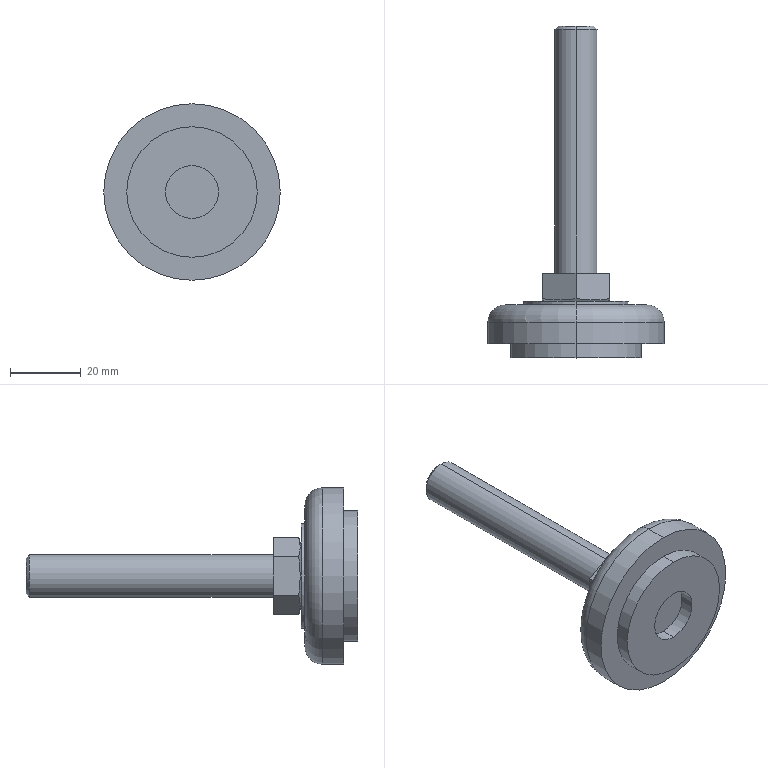Part | STEP file | FJSN12_70pad | 1 solid | 29 faces | box 50 x 94 x 50 mm | volume 35453 mm3 | plane 13 | cylinder 10 | cone 4 | torus 2 | commonest cylinder face diameters 12 x2 15 x2 29.75 x2 37 x2 50 x2
STEP:
#1=CARTESIAN_POINT('',(0.,24.,6.));
#2=VERTEX_POINT('',#1);
#3=CARTESIAN_POINT('',(0.,24.,-6.));
#4=VERTEX_POINT('',#3);
#5=CARTESIAN_POINT('',(0.,24.,0.));
#6=DIRECTION('',(0.,1.,0.));
#7=DIRECTION('',(0.,0.,1.));
#8=AXIS2_PLACEMENT_3D('',#5,#6,#7);
#9=CIRCLE('',#8,6.);
#10=EDGE_CURVE('',#2,#4,#9,.T.);
#11=ORIENTED_EDGE('',*,*,#10,.T.);
#12=CARTESIAN_POINT('',(0.,93.053,-6.));
#13=VERTEX_POINT('',#12);
#14=CARTESIAN_POINT('',(0.,0.,-6.));
#15=DIRECTION('',(0.,1.,0.));
#16=VECTOR('',#15,1000.);
#17=LINE('',#14,#16);
#18=EDGE_CURVE('',#4,#13,#17,.T.);
#19=ORIENTED_EDGE('',*,*,#18,.T.);
#20=CARTESIAN_POINT('',(0.,93.053,6.));
#21=VERTEX_POINT('',#20);
#22=CARTESIAN_POINT('',(0.,93.053,0.));
#23=DIRECTION('',(0.,1.,0.));
#24=DIRECTION('',(0.,0.,1.));
#25=AXIS2_PLACEMENT_3D('',#22,#23,#24);
#26=CIRCLE('',#25,6.);
#27=EDGE_CURVE('',#21,#13,#26,.T.);
#28=ORIENTED_EDGE('',*,*,#27,.F.);
#29=CARTESIAN_POINT('',(0.,0.,6.));
#30=DIRECTION('',(0.,1.,0.));
#31=VECTOR('',#30,1000.);
#32=LINE('',#29,#31);
#33=EDGE_CURVE('',#2,#21,#32,.T.);
#34=ORIENTED_EDGE('',*,*,#33,.F.);
#35=EDGE_LOOP('',(#11,#19,#28,#34));
#36=FACE_OUTER_BOUND('',#35,.T.);
#37=CARTESIAN_POINT('',(0.,0.,0.));
#38=DIRECTION('',(0.,1.,0.));
#39=DIRECTION('',(0.,0.,1.));
#40=AXIS2_PLACEMENT_3D('',#37,#38,#39);
#41=CYLINDRICAL_SURFACE('',#40,6.);
#42=ADVANCED_FACE('',(#36),#41,.T.);
#43=CARTESIAN_POINT('',(0.,94.,5.053));
#44=VERTEX_POINT('',#43);
#45=CARTESIAN_POINT('',(0.,94.,-5.053));
#46=VERTEX_POINT('',#45);
#47=CARTESIAN_POINT('',(0.,94.,0.));
#48=DIRECTION('',(0.,1.,0.));
#49=DIRECTION('',(0.,0.,1.));
#50=AXIS2_PLACEMENT_3D('',#47,#48,#49);
#51=CIRCLE('',#50,5.053);
#52=EDGE_CURVE('',#44,#46,#51,.T.);
#53=ORIENTED_EDGE('',*,*,#52,.F.);
#54=CARTESIAN_POINT('',(0.,93.053,6.));
#55=DIRECTION('',(0.,-0.7071,0.7071));
#56=VECTOR('',#55,1000.);
#57=LINE('',#54,#56);
#58=EDGE_CURVE('',#44,#21,#57,.T.);
#59=ORIENTED_EDGE('',*,*,#58,.T.);
#60=ORIENTED_EDGE('',*,*,#27,.T.);
#61=CARTESIAN_POINT('',(0.,93.053,-6.));
#62=DIRECTION('',(0.,-0.7071,-0.7071));
#63=VECTOR('',#62,1000.);
#64=LINE('',#61,#63);
#65=EDGE_CURVE('',#46,#13,#64,.T.);
#66=ORIENTED_EDGE('',*,*,#65,.F.);
#67=EDGE_LOOP('',(#53,#59,#60,#66));
#68=FACE_OUTER_BOUND('',#67,.T.);
#69=CARTESIAN_POINT('',(0.,93.053,0.));
#70=DIRECTION('',(0.,-1.,0.));
#71=DIRECTION('',(0.,0.,-1.));
#72=AXIS2_PLACEMENT_3D('',#69,#70,#71);
#73=CONICAL_SURFACE('',#72,6.,0.7854);
#74=ADVANCED_FACE('',(#68),#73,.T.);
#75=CARTESIAN_POINT('',(0.,0.,-7.5));
#76=VERTEX_POINT('',#75);
#77=CARTESIAN_POINT('',(0.,0.,7.5));
#78=VERTEX_POINT('',#77);
#79=CARTESIAN_POINT('',(0.,0.,0.));
#80=DIRECTION('',(0.,1.,0.));
#81=DIRECTION('',(0.,0.,1.));
#82=AXIS2_PLACEMENT_3D('',#79,#80,#81);
#83=CIRCLE('',#82,7.5);
#84=EDGE_CURVE('',#76,#78,#83,.T.);
#85=ORIENTED_EDGE('',*,*,#84,.F.);
#86=CARTESIAN_POINT('',(0.,4.,-7.5));
#87=VERTEX_POINT('',#86);
#88=CARTESIAN_POINT('',(0.,0.,-7.5));
#89=DIRECTION('',(0.,1.,0.));
#90=VECTOR('',#89,1000.);
#91=LINE('',#88,#90);
#92=EDGE_CURVE('',#76,#87,#91,.T.);
#93=ORIENTED_EDGE('',*,*,#92,.T.);
#94=CARTESIAN_POINT('',(0.,4.,7.5));
#95=VERTEX_POINT('',#94);
#96=CARTESIAN_POINT('',(0.,4.,0.));
#97=DIRECTION('',(0.,1.,0.));
#98=DIRECTION('',(0.,0.,1.));
#99=AXIS2_PLACEMENT_3D('',#96,#97,#98);
#100=CIRCLE('',#99,7.5);
#101=EDGE_CURVE('',#87,#95,#100,.T.);
#102=ORIENTED_EDGE('',*,*,#101,.T.);
#103=CARTESIAN_POINT('',(0.,0.,7.5));
#104=DIRECTION('',(0.,1.,0.));
#105=VECTOR('',#104,1000.);
#106=LINE('',#103,#105);
#107=EDGE_CURVE('',#78,#95,#106,.T.);
#108=ORIENTED_EDGE('',*,*,#107,.F.);
#109=EDGE_LOOP('',(#85,#93,#102,#108));
#110=FACE_OUTER_BOUND('',#109,.T.);
#111=CARTESIAN_POINT('',(0.,0.,0.));
#112=DIRECTION('',(0.,1.,0.));
#113=DIRECTION('',(0.,0.,1.));
#114=AXIS2_PLACEMENT_3D('',#111,#112,#113);
#115=CYLINDRICAL_SURFACE('',#114,7.5);
#116=ADVANCED_FACE('',(#110),#115,.F.);
#117=CARTESIAN_POINT('',(0.,0.,18.5));
#118=VERTEX_POINT('',#117);
#119=CARTESIAN_POINT('',(0.,0.,-18.5));
#120=VERTEX_POINT('',#119);
#121=CARTESIAN_POINT('',(0.,0.,0.));
#122=DIRECTION('',(0.,1.,0.));
#123=DIRECTION('',(0.,0.,1.));
#124=AXIS2_PLACEMENT_3D('',#121,#122,#123);
#125=CIRCLE('',#124,18.5);
#126=EDGE_CURVE('',#118,#120,#125,.T.);
#127=ORIENTED_EDGE('',*,*,#126,.T.);
#128=CARTESIAN_POINT('',(0.,4.,-18.5));
#129=VERTEX_POINT('',#128);
#130=CARTESIAN_POINT('',(0.,0.,-18.5));
#131=DIRECTION('',(0.,1.,0.));
#132=VECTOR('',#131,1000.);
#133=LINE('',#130,#132);
#134=EDGE_CURVE('',#120,#129,#133,.T.);
#135=ORIENTED_EDGE('',*,*,#134,.T.);
#136=CARTESIAN_POINT('',(0.,4.,18.5));
#137=VERTEX_POINT('',#136);
#138=CARTESIAN_POINT('',(0.,4.,0.));
#139=DIRECTION('',(0.,1.,0.));
#140=DIRECTION('',(0.,0.,1.));
#141=AXIS2_PLACEMENT_3D('',#138,#139,#140);
#142=CIRCLE('',#141,18.5);
#143=EDGE_CURVE('',#137,#129,#142,.T.);
#144=ORIENTED_EDGE('',*,*,#143,.F.);
#145=CARTESIAN_POINT('',(0.,0.,18.5));
#146=DIRECTION('',(0.,1.,0.));
#147=VECTOR('',#146,1000.);
#148=LINE('',#145,#147);
#149=EDGE_CURVE('',#118,#137,#148,.T.);
#150=ORIENTED_EDGE('',*,*,#149,.F.);
#151=EDGE_LOOP('',(#127,#135,#144,#150));
#152=FACE_OUTER_BOUND('',#151,.T.);
#153=CARTESIAN_POINT('',(0.,0.,0.));
#154=DIRECTION('',(0.,1.,0.));
#155=DIRECTION('',(0.,0.,1.));
#156=AXIS2_PLACEMENT_3D('',#153,#154,#155);
#157=CYLINDRICAL_SURFACE('',#156,18.5);
#158=ADVANCED_FACE('',(#152),#157,.T.);
#159=CARTESIAN_POINT('',(0.,4.,25.));
#160=VERTEX_POINT('',#159);
#161=CARTESIAN_POINT('',(0.,4.,-25.));
#162=VERTEX_POINT('',#161);
#163=CARTESIAN_POINT('',(0.,4.,0.));
#164=DIRECTION('',(0.,1.,0.));
#165=DIRECTION('',(0.,0.,1.));
#166=AXIS2_PLACEMENT_3D('',#163,#164,#165);
#167=CIRCLE('',#166,25.);
#168=EDGE_CURVE('',#160,#162,#167,.T.);
#169=ORIENTED_EDGE('',*,*,#168,.T.);
#170=CARTESIAN_POINT('',(0.,10.,-25.));
#171=VERTEX_POINT('',#170);
#172=CARTESIAN_POINT('',(0.,0.,-25.));
#173=DIRECTION('',(0.,1.,0.));
#174=VECTOR('',#173,1000.);
#175=LINE('',#172,#174);
#176=EDGE_CURVE('',#162,#171,#175,.T.);
#177=ORIENTED_EDGE('',*,*,#176,.T.);
#178=CARTESIAN_POINT('',(0.,10.,25.));
#179=VERTEX_POINT('',#178);
#180=CARTESIAN_POINT('',(0.,10.,0.));
#181=DIRECTION('',(0.,1.,0.));
#182=DIRECTION('',(0.,0.,1.));
#183=AXIS2_PLACEMENT_3D('',#180,#181,#182);
#184=CIRCLE('',#183,25.);
#185=EDGE_CURVE('',#179,#171,#184,.T.);
#186=ORIENTED_EDGE('',*,*,#185,.F.);
#187=CARTESIAN_POINT('',(0.,0.,25.));
#188=DIRECTION('',(0.,1.,0.));
#189=VECTOR('',#188,1000.);
#190=LINE('',#187,#189);
#191=EDGE_CURVE('',#160,#179,#190,.T.);
#192=ORIENTED_EDGE('',*,*,#191,.F.);
#193=EDGE_LOOP('',(#169,#177,#186,#192));
#194=FACE_OUTER_BOUND('',#193,.T.);
#195=CARTESIAN_POINT('',(0.,0.,0.));
#196=DIRECTION('',(0.,1.,0.));
#197=DIRECTION('',(0.,0.,1.));
#198=AXIS2_PLACEMENT_3D('',#195,#196,#197);
#199=CYLINDRICAL_SURFACE('',#198,25.);
#200=ADVANCED_FACE('',(#194),#199,.T.);
#201=ORIENTED_EDGE('',*,*,#185,.T.);
#202=CARTESIAN_POINT('',(0.,15.,-20.));
#203=VERTEX_POINT('',#202);
#204=CARTESIAN_POINT('',(0.,10.,-20.));
#205=DIRECTION('',(1.,0.,0.));
#206=DIRECTION('',(0.,0.,-1.));
#207=AXIS2_PLACEMENT_3D('',#204,#205,#206);
#208=CIRCLE('',#207,5.);
#209=EDGE_CURVE('',#171,#203,#208,.T.);
#210=ORIENTED_EDGE('',*,*,#209,.T.);
#211=CARTESIAN_POINT('',(0.,15.,20.));
#212=VERTEX_POINT('',#211);
#213=CARTESIAN_POINT('',(0.,15.,0.));
#214=DIRECTION('',(0.,1.,0.));
#215=DIRECTION('',(0.,0.,1.));
#216=AXIS2_PLACEMENT_3D('',#213,#214,#215);
#217=CIRCLE('',#216,20.);
#218=EDGE_CURVE('',#212,#203,#217,.T.);
#219=ORIENTED_EDGE('',*,*,#218,.F.);
#220=CARTESIAN_POINT('',(0.,10.,20.));
#221=DIRECTION('',(-1.,0.,0.));
#222=DIRECTION('',(0.,0.,1.));
#223=AXIS2_PLACEMENT_3D('',#220,#221,#222);
#224=CIRCLE('',#223,5.);
#225=EDGE_CURVE('',#179,#212,#224,.T.);
#226=ORIENTED_EDGE('',*,*,#225,.F.);
#227=EDGE_LOOP('',(#201,#210,#219,#226));
#228=FACE_OUTER_BOUND('',#227,.T.);
#229=CARTESIAN_POINT('',(0.,10.,0.));
#230=DIRECTION('',(0.,1.,0.));
#231=DIRECTION('',(0.,0.,1.));
#232=AXIS2_PLACEMENT_3D('',#229,#230,#231);
#233=TOROIDAL_SURFACE('',#232,20.,5.);
#234=ADVANCED_FACE('',(#228),#233,.T.);
#235=CARTESIAN_POINT('',(0.,15.,14.875));
#236=VERTEX_POINT('',#235);
#237=CARTESIAN_POINT('',(0.,15.,-14.875));
#238=VERTEX_POINT('',#237);
#239=CARTESIAN_POINT('',(0.,15.,0.));
#240=DIRECTION('',(0.,1.,0.));
#241=DIRECTION('',(0.,0.,1.));
#242=AXIS2_PLACEMENT_3D('',#239,#240,#241);
#243=CIRCLE('',#242,14.875);
#244=EDGE_CURVE('',#236,#238,#243,.T.);
#245=ORIENTED_EDGE('',*,*,#244,.T.);
#246=CARTESIAN_POINT('',(0.,16.,-14.875));
#247=VERTEX_POINT('',#246);
#248=CARTESIAN_POINT('',(0.,0.,-14.875));
#249=DIRECTION('',(0.,1.,0.));
#250=VECTOR('',#249,1000.);
#251=LINE('',#248,#250);
#252=EDGE_CURVE('',#238,#247,#251,.T.);
#253=ORIENTED_EDGE('',*,*,#252,.T.);
#254=CARTESIAN_POINT('',(0.,16.,14.875));
#255=VERTEX_POINT('',#254);
#256=CARTESIAN_POINT('',(0.,16.,0.));
#257=DIRECTION('',(0.,1.,0.));
#258=DIRECTION('',(0.,0.,1.));
#259=AXIS2_PLACEMENT_3D('',#256,#257,#258);
#260=CIRCLE('',#259,14.875);
#261=EDGE_CURVE('',#255,#247,#260,.T.);
#262=ORIENTED_EDGE('',*,*,#261,.F.);
#263=CARTESIAN_POINT('',(0.,0.,14.875));
#264=DIRECTION('',(0.,1.,0.));
#265=VECTOR('',#264,1000.);
#266=LINE('',#263,#265);
#267=EDGE_CURVE('',#236,#255,#266,.T.);
#268=ORIENTED_EDGE('',*,*,#267,.F.);
#269=EDGE_LOOP('',(#245,#253,#262,#268));
#270=FACE_OUTER_BOUND('',#269,.T.);
#271=CARTESIAN_POINT('',(0.,0.,0.));
#272=DIRECTION('',(0.,1.,0.));
#273=DIRECTION('',(0.,0.,1.));
#274=AXIS2_PLACEMENT_3D('',#271,#272,#273);
#275=CYLINDRICAL_SURFACE('',#274,14.875);
#276=ADVANCED_FACE('',(#270),#275,.T.);
#277=CARTESIAN_POINT('',(0.,16.,8.));
#278=VERTEX_POINT('',#277);
#279=CARTESIAN_POINT('',(0.,16.,-8.));
#280=VERTEX_POINT('',#279);
#281=CARTESIAN_POINT('',(0.,16.,0.));
#282=DIRECTION('',(0.,1.,0.));
#283=DIRECTION('',(0.,0.,1.));
#284=AXIS2_PLACEMENT_3D('',#281,#282,#283);
#285=CIRCLE('',#284,8.);
#286=EDGE_CURVE('',#278,#280,#285,.T.);
#287=ORIENTED_EDGE('',*,*,#286,.T.);
#288=CARTESIAN_POINT('',(0.,16.766,-10.97));
#289=VERTEX_POINT('',#288);
#290=CARTESIAN_POINT('',(0.,16.,-8.));
#291=DIRECTION('',(0.,0.2499,-0.9683));
#292=VECTOR('',#291,1000.);
#293=LINE('',#290,#292);
#294=EDGE_CURVE('',#280,#289,#293,.T.);
#295=ORIENTED_EDGE('',*,*,#294,.T.);
#296=CARTESIAN_POINT('',(9.5,16.766,-5.485));
#297=VERTEX_POINT('',#296);
#298=CARTESIAN_POINT('',(0.,16.766,-10.97));
#299=CARTESIAN_POINT('',(0.7917,16.648,-10.513));
#300=CARTESIAN_POINT('',(1.583,16.553,-10.056));
#301=CARTESIAN_POINT('',(3.167,16.422,-9.141));
#302=CARTESIAN_POINT('',(4.75,16.352,-8.227));
#303=CARTESIAN_POINT('',(6.333,16.422,-7.313));
#304=CARTESIAN_POINT('',(7.917,16.553,-6.399));
#305=CARTESIAN_POINT('',(8.708,16.648,-5.942));
#306=CARTESIAN_POINT('',(9.5,16.766,-5.485));
#307=B_SPLINE_CURVE_WITH_KNOTS('',3,(#298,#299,#300,#301,#302,#303,#304,#305,#306),.UNSPECIFIED.,.F.,.F.,(4,2,1,2,4),(0.000000231,0.002743,0.005485,0.008227,0.01097),.UNSPECIFIED.);
#308=EDGE_CURVE('',#289,#297,#307,.T.);
#309=ORIENTED_EDGE('',*,*,#308,.T.);
#310=CARTESIAN_POINT('',(9.5,16.766,5.485));
#311=VERTEX_POINT('',#310);
#312=CARTESIAN_POINT('',(9.5,16.766,-5.485));
#313=CARTESIAN_POINT('',(9.5,16.649,-4.572));
#314=CARTESIAN_POINT('',(9.5,16.552,-3.654));
#315=CARTESIAN_POINT('',(9.5,16.421,-1.821));
#316=CARTESIAN_POINT('',(9.5,16.387,-0.9056));
#317=CARTESIAN_POINT('',(9.5,16.387,0.9233));
#318=CARTESIAN_POINT('',(9.5,16.422,1.837));
#319=CARTESIAN_POINT('',(9.5,16.553,3.662));
#320=CARTESIAN_POINT('',(9.5,16.649,4.574));
#321=CARTESIAN_POINT('',(9.5,16.766,5.485));
#322=B_SPLINE_CURVE_WITH_KNOTS('',3,(#312,#313,#314,#315,#316,#317,#318,#319,#320,#321),.UNSPECIFIED.,.F.,.F.,(4,2,2,2,4),(0.009151,0.01191,0.01467,0.01743,0.02019),.UNSPECIFIED.);
#323=EDGE_CURVE('',#297,#311,#322,.T.);
#324=ORIENTED_EDGE('',*,*,#323,.T.);
#325=CARTESIAN_POINT('',(0.,16.766,10.97));
#326=VERTEX_POINT('',#325);
#327=CARTESIAN_POINT('',(9.5,16.766,5.485));
#328=CARTESIAN_POINT('',(8.708,16.648,5.942));
#329=CARTESIAN_POINT('',(7.917,16.553,6.399));
#330=CARTESIAN_POINT('',(6.333,16.422,7.313));
#331=CARTESIAN_POINT('',(4.75,16.352,8.227));
#332=CARTESIAN_POINT('',(3.167,16.422,9.141));
#333=CARTESIAN_POINT('',(1.583,16.553,10.056));
#334=CARTESIAN_POINT('',(0.7917,16.648,10.513));
#335=CARTESIAN_POINT('',(0.,16.766,10.97));
#336=B_SPLINE_CURVE_WITH_KNOTS('',3,(#327,#328,#329,#330,#331,#332,#333,#334,#335),.UNSPECIFIED.,.F.,.F.,(4,2,1,2,4),(0.000000231,0.002743,0.005485,0.008227,0.01097),.UNSPECIFIED.);
#337=EDGE_CURVE('',#311,#326,#336,.T.);
#338=ORIENTED_EDGE('',*,*,#337,.T.);
#339=CARTESIAN_POINT('',(0.,16.,8.));
#340=DIRECTION('',(0.,0.2499,0.9683));
#341=VECTOR('',#340,1000.);
#342=LINE('',#339,#341);
#343=EDGE_CURVE('',#278,#326,#342,.T.);
#344=ORIENTED_EDGE('',*,*,#343,.F.);
#345=EDGE_LOOP('',(#287,#295,#309,#324,#338,#344));
#346=FACE_OUTER_BOUND('',#345,.T.);
#347=CARTESIAN_POINT('',(0.,16.,0.));
#348=DIRECTION('',(0.,1.,0.));
#349=DIRECTION('',(0.,0.,1.));
#350=AXIS2_PLACEMENT_3D('',#347,#348,#349);
#351=CONICAL_SURFACE('',#350,8.,1.318);
#352=ADVANCED_FACE('',(#346),#351,.T.);
#353=ORIENTED_EDGE('',*,*,#294,.F.);
#354=CARTESIAN_POINT('',(0.,16.,0.));
#355=DIRECTION('',(0.,1.,0.));
#356=DIRECTION('',(0.,0.,1.));
#357=AXIS2_PLACEMENT_3D('',#354,#355,#356);
#358=CIRCLE('',#357,8.);
#359=EDGE_CURVE('',#280,#278,#358,.T.);
#360=ORIENTED_EDGE('',*,*,#359,.T.);
#361=ORIENTED_EDGE('',*,*,#343,.T.);
#362=CARTESIAN_POINT('',(-9.5,16.766,5.485));
#363=VERTEX_POINT('',#362);
#364=CARTESIAN_POINT('',(0.,16.766,10.97));
#365=CARTESIAN_POINT('',(-0.7917,16.648,10.513));
#366=CARTESIAN_POINT('',(-1.583,16.553,10.056));
#367=CARTESIAN_POINT('',(-3.167,16.422,9.141));
#368=CARTESIAN_POINT('',(-4.75,16.352,8.227));
#369=CARTESIAN_POINT('',(-6.333,16.422,7.313));
#370=CARTESIAN_POINT('',(-7.917,16.553,6.399));
#371=CARTESIAN_POINT('',(-8.708,16.648,5.942));
#372=CARTESIAN_POINT('',(-9.5,16.766,5.485));
#373=B_SPLINE_CURVE_WITH_KNOTS('',3,(#364,#365,#366,#367,#368,#369,#370,#371,#372),.UNSPECIFIED.,.F.,.F.,(4,2,1,2,4),(0.000000231,0.002743,0.005485,0.008227,0.01097),.UNSPECIFIED.);
#374=EDGE_CURVE('',#326,#363,#373,.T.);
#375=ORIENTED_EDGE('',*,*,#374,.T.);
#376=CARTESIAN_POINT('',(-9.5,16.766,-5.485));
#377=VERTEX_POINT('',#376);
#378=CARTESIAN_POINT('',(-9.5,16.766,5.485));
#379=CARTESIAN_POINT('',(-9.5,16.649,4.574));
#380=CARTESIAN_POINT('',(-9.5,16.553,3.662));
#381=CARTESIAN_POINT('',(-9.5,16.422,1.837));
#382=CARTESIAN_POINT('',(-9.5,16.387,0.9233));
#383=CARTESIAN_POINT('',(-9.5,16.387,-0.9056));
#384=CARTESIAN_POINT('',(-9.5,16.421,-1.821));
#385=CARTESIAN_POINT('',(-9.5,16.552,-3.654));
#386=CARTESIAN_POINT('',(-9.5,16.649,-4.572));
#387=CARTESIAN_POINT('',(-9.5,16.766,-5.485));
#388=B_SPLINE_CURVE_WITH_KNOTS('',3,(#378,#379,#380,#381,#382,#383,#384,#385,#386,#387),.UNSPECIFIED.,.F.,.F.,(4,2,2,2,4),(0.02104,0.02379,0.02655,0.0293,0.03206),.UNSPECIFIED.);
#389=EDGE_CURVE('',#363,#377,#388,.T.);
#390=ORIENTED_EDGE('',*,*,#389,.T.);
#391=CARTESIAN_POINT('',(-9.5,16.766,-5.485));
#392=CARTESIAN_POINT('',(-8.708,16.648,-5.942));
#393=CARTESIAN_POINT('',(-7.917,16.553,-6.399));
#394=CARTESIAN_POINT('',(-6.333,16.422,-7.313));
#395=CARTESIAN_POINT('',(-4.75,16.352,-8.227));
#396=CARTESIAN_POINT('',(-3.167,16.422,-9.141));
#397=CARTESIAN_POINT('',(-1.583,16.553,-10.056));
#398=CARTESIAN_POINT('',(-0.7917,16.648,-10.513));
#399=CARTESIAN_POINT('',(0.,16.766,-10.97));
#400=B_SPLINE_CURVE_WITH_KNOTS('',3,(#391,#392,#393,#394,#395,#396,#397,#398,#399),.UNSPECIFIED.,.F.,.F.,(4,2,1,2,4),(0.000000231,0.002743,0.005485,0.008227,0.01097),.UNSPECIFIED.);
#401=EDGE_CURVE('',#377,#289,#400,.T.);
#402=ORIENTED_EDGE('',*,*,#401,.T.);
#403=EDGE_LOOP('',(#353,#360,#361,#375,#390,#402));
#404=FACE_OUTER_BOUND('',#403,.T.);
#405=CARTESIAN_POINT('',(0.,16.,0.));
#406=DIRECTION('',(0.,1.,0.));
#407=DIRECTION('',(0.,0.,1.));
#408=AXIS2_PLACEMENT_3D('',#405,#406,#407);
#409=CONICAL_SURFACE('',#408,8.,1.318);
#410=ADVANCED_FACE('',(#404),#409,.T.);
#411=ORIENTED_EDGE('',*,*,#286,.F.);
#412=ORIENTED_EDGE('',*,*,#359,.F.);
#413=EDGE_LOOP('',(#411,#412));
#414=FACE_BOUND('',#413,.T.);
#415=ORIENTED_EDGE('',*,*,#261,.T.);
#416=CARTESIAN_POINT('',(0.,16.,0.));
#417=DIRECTION('',(0.,1.,0.));
#418=DIRECTION('',(0.,0.,1.));
#419=AXIS2_PLACEMENT_3D('',#416,#417,#418);
#420=CIRCLE('',#419,14.875);
#421=EDGE_CURVE('',#247,#255,#420,.T.);
#422=ORIENTED_EDGE('',*,*,#421,.T.);
#423=EDGE_LOOP('',(#415,#422));
#424=FACE_OUTER_BOUND('',#423,.T.);
#425=CARTESIAN_POINT('',(8.,16.,0.));
#426=DIRECTION('',(0.,-1.,0.));
#427=DIRECTION('',(0.,0.,-1.));
#428=AXIS2_PLACEMENT_3D('',#425,#426,#427);
#429=PLANE('',#428);
#430=ADVANCED_FACE('',(#414,#424),#429,.F.);
#431=ORIENTED_EDGE('',*,*,#252,.F.);
#432=CARTESIAN_POINT('',(0.,15.,0.));
#433=DIRECTION('',(0.,1.,0.));
#434=DIRECTION('',(0.,0.,1.));
#435=AXIS2_PLACEMENT_3D('',#432,#433,#434);
#436=CIRCLE('',#435,14.875);
#437=EDGE_CURVE('',#238,#236,#436,.T.);
#438=ORIENTED_EDGE('',*,*,#437,.T.);
#439=ORIENTED_EDGE('',*,*,#267,.T.);
#440=ORIENTED_EDGE('',*,*,#421,.F.);
#441=EDGE_LOOP('',(#431,#438,#439,#440));
#442=FACE_OUTER_BOUND('',#441,.T.);
#443=CARTESIAN_POINT('',(0.,0.,0.));
#444=DIRECTION('',(0.,1.,0.));
#445=DIRECTION('',(0.,0.,1.));
#446=AXIS2_PLACEMENT_3D('',#443,#444,#445);
#447=CYLINDRICAL_SURFACE('',#446,14.875);
#448=ADVANCED_FACE('',(#442),#447,.T.);
#449=ORIENTED_EDGE('',*,*,#244,.F.);
#450=ORIENTED_EDGE('',*,*,#437,.F.);
#451=EDGE_LOOP('',(#449,#450));
#452=FACE_BOUND('',#451,.T.);
#453=ORIENTED_EDGE('',*,*,#218,.T.);
#454=CARTESIAN_POINT('',(0.,15.,0.));
#455=DIRECTION('',(0.,1.,0.));
#456=DIRECTION('',(0.,0.,1.));
#457=AXIS2_PLACEMENT_3D('',#454,#455,#456);
#458=CIRCLE('',#457,20.);
#459=EDGE_CURVE('',#203,#212,#458,.T.);
#460=ORIENTED_EDGE('',*,*,#459,.T.);
#461=EDGE_LOOP('',(#453,#460));
#462=FACE_OUTER_BOUND('',#461,.T.);
#463=CARTESIAN_POINT('',(14.875,15.,0.));
#464=DIRECTION('',(0.,-1.,0.));
#465=DIRECTION('',(0.,0.,-1.));
#466=AXIS2_PLACEMENT_3D('',#463,#464,#465);
#467=PLANE('',#466);
#468=ADVANCED_FACE('',(#452,#462),#467,.F.);
#469=ORIENTED_EDGE('',*,*,#209,.F.);
#470=CARTESIAN_POINT('',(0.,10.,0.));
#471=DIRECTION('',(0.,1.,0.));
#472=DIRECTION('',(0.,0.,1.));
#473=AXIS2_PLACEMENT_3D('',#470,#471,#472);
#474=CIRCLE('',#473,25.);
#475=EDGE_CURVE('',#171,#179,#474,.T.);
#476=ORIENTED_EDGE('',*,*,#475,.T.);
#477=ORIENTED_EDGE('',*,*,#225,.T.);
#478=ORIENTED_EDGE('',*,*,#459,.F.);
#479=EDGE_LOOP('',(#469,#476,#477,#478));
#480=FACE_OUTER_BOUND('',#479,.T.);
#481=CARTESIAN_POINT('',(0.,10.,0.));
#482=DIRECTION('',(0.,1.,0.));
#483=DIRECTION('',(0.,0.,1.));
#484=AXIS2_PLACEMENT_3D('',#481,#482,#483);
#485=TOROIDAL_SURFACE('',#484,20.,5.);
#486=ADVANCED_FACE('',(#480),#485,.T.);
#487=ORIENTED_EDGE('',*,*,#176,.F.);
#488=CARTESIAN_POINT('',(0.,4.,0.));
#489=DIRECTION('',(0.,1.,0.));
#490=DIRECTION('',(0.,0.,1.));
#491=AXIS2_PLACEMENT_3D('',#488,#489,#490);
#492=CIRCLE('',#491,25.);
#493=EDGE_CURVE('',#162,#160,#492,.T.);
#494=ORIENTED_EDGE('',*,*,#493,.T.);
#495=ORIENTED_EDGE('',*,*,#191,.T.);
#496=ORIENTED_EDGE('',*,*,#475,.F.);
#497=EDGE_LOOP('',(#487,#494,#495,#496));
#498=FACE_OUTER_BOUND('',#497,.T.);
#499=CARTESIAN_POINT('',(0.,0.,0.));
#500=DIRECTION('',(0.,1.,0.));
#501=DIRECTION('',(0.,0.,1.));
#502=AXIS2_PLACEMENT_3D('',#499,#500,#501);
#503=CYLINDRICAL_SURFACE('',#502,25.);
#504=ADVANCED_FACE('',(#498),#503,.T.);
#505=ORIENTED_EDGE('',*,*,#168,.F.);
#506=ORIENTED_EDGE('',*,*,#493,.F.);
#507=EDGE_LOOP('',(#505,#506));
#508=FACE_OUTER_BOUND('',#507,.T.);
#509=ORIENTED_EDGE('',*,*,#143,.T.);
#510=CARTESIAN_POINT('',(0.,4.,0.));
#511=DIRECTION('',(0.,1.,0.));
#512=DIRECTION('',(0.,0.,1.));
#513=AXIS2_PLACEMENT_3D('',#510,#511,#512);
#514=CIRCLE('',#513,18.5);
#515=EDGE_CURVE('',#129,#137,#514,.T.);
#516=ORIENTED_EDGE('',*,*,#515,.T.);
#517=EDGE_LOOP('',(#509,#516));
#518=FACE_BOUND('',#517,.T.);
#519=CARTESIAN_POINT('',(25.,4.,0.));
#520=DIRECTION('',(0.,1.,0.));
#521=DIRECTION('',(0.,0.,1.));
#522=AXIS2_PLACEMENT_3D('',#519,#520,#521);
#523=PLANE('',#522);
#524=ADVANCED_FACE('',(#508,#518),#523,.F.);
#525=ORIENTED_EDGE('',*,*,#134,.F.);
#526=CARTESIAN_POINT('',(0.,0.,0.));
#527=DIRECTION('',(0.,1.,0.));
#528=DIRECTION('',(0.,0.,1.));
#529=AXIS2_PLACEMENT_3D('',#526,#527,#528);
#530=CIRCLE('',#529,18.5);
#531=EDGE_CURVE('',#120,#118,#530,.T.);
#532=ORIENTED_EDGE('',*,*,#531,.T.);
#533=ORIENTED_EDGE('',*,*,#149,.T.);
#534=ORIENTED_EDGE('',*,*,#515,.F.);
#535=EDGE_LOOP('',(#525,#532,#533,#534));
#536=FACE_OUTER_BOUND('',#535,.T.);
#537=CARTESIAN_POINT('',(0.,0.,0.));
#538=DIRECTION('',(0.,1.,0.));
#539=DIRECTION('',(0.,0.,1.));
#540=AXIS2_PLACEMENT_3D('',#537,#538,#539);
#541=CYLINDRICAL_SURFACE('',#540,18.5);
#542=ADVANCED_FACE('',(#536),#541,.T.);
#543=ORIENTED_EDGE('',*,*,#126,.F.);
#544=ORIENTED_EDGE('',*,*,#531,.F.);
#545=EDGE_LOOP('',(#543,#544));
#546=FACE_OUTER_BOUND('',#545,.T.);
#547=CARTESIAN_POINT('',(0.,0.,0.));
#548=DIRECTION('',(0.,1.,0.));
#549=DIRECTION('',(0.,0.,1.));
#550=AXIS2_PLACEMENT_3D('',#547,#548,#549);
#551=CIRCLE('',#550,7.5);
#552=EDGE_CURVE('',#78,#76,#551,.T.);
#553=ORIENTED_EDGE('',*,*,#552,.T.);
#554=ORIENTED_EDGE('',*,*,#84,.T.);
#555=EDGE_LOOP('',(#553,#554));
#556=FACE_BOUND('',#555,.T.);
#557=CARTESIAN_POINT('',(18.5,0.,0.));
#558=DIRECTION('',(0.,1.,0.));
#559=DIRECTION('',(0.,0.,1.));
#560=AXIS2_PLACEMENT_3D('',#557,#558,#559);
#561=PLANE('',#560);
#562=ADVANCED_FACE('',(#546,#556),#561,.F.);
#563=ORIENTED_EDGE('',*,*,#92,.F.);
#564=ORIENTED_EDGE('',*,*,#552,.F.);
#565=ORIENTED_EDGE('',*,*,#107,.T.);
#566=CARTESIAN_POINT('',(0.,4.,0.));
#567=DIRECTION('',(0.,1.,0.));
#568=DIRECTION('',(0.,0.,1.));
#569=AXIS2_PLACEMENT_3D('',#566,#567,#568);
#570=CIRCLE('',#569,7.5);
#571=EDGE_CURVE('',#95,#87,#570,.T.);
#572=ORIENTED_EDGE('',*,*,#571,.T.);
#573=EDGE_LOOP('',(#563,#564,#565,#572));
#574=FACE_OUTER_BOUND('',#573,.T.);
#575=CARTESIAN_POINT('',(0.,0.,0.));
#576=DIRECTION('',(0.,1.,0.));
#577=DIRECTION('',(0.,0.,1.));
#578=AXIS2_PLACEMENT_3D('',#575,#576,#577);
#579=CYLINDRICAL_SURFACE('',#578,7.5);
#580=ADVANCED_FACE('',(#574),#579,.F.);
#581=ORIENTED_EDGE('',*,*,#571,.F.);
#582=ORIENTED_EDGE('',*,*,#101,.F.);
#583=EDGE_LOOP('',(#581,#582));
#584=FACE_OUTER_BOUND('',#583,.T.);
#585=CARTESIAN_POINT('',(7.5,4.,0.));
#586=DIRECTION('',(0.,1.,0.));
#587=DIRECTION('',(0.,0.,1.));
#588=AXIS2_PLACEMENT_3D('',#585,#586,#587);
#589=PLANE('',#588);
#590=ADVANCED_FACE('',(#584),#589,.F.);
#591=CARTESIAN_POINT('',(0.,24.,-10.97));
#592=VERTEX_POINT('',#591);
#593=CARTESIAN_POINT('',(0.,25.,-10.97));
#594=DIRECTION('',(0.,-1.,0.));
#595=VECTOR('',#594,1000.);
#596=LINE('',#593,#595);
#597=EDGE_CURVE('',#592,#289,#596,.T.);
#598=ORIENTED_EDGE('',*,*,#597,.T.);
#599=ORIENTED_EDGE('',*,*,#401,.F.);
#600=CARTESIAN_POINT('',(-9.5,24.,-5.485));
#601=VERTEX_POINT('',#600);
#602=CARTESIAN_POINT('',(-9.5,25.,-5.485));
#603=DIRECTION('',(0.,-1.,0.));
#604=VECTOR('',#603,1000.);
#605=LINE('',#602,#604);
#606=EDGE_CURVE('',#601,#377,#605,.T.);
#607=ORIENTED_EDGE('',*,*,#606,.F.);
#608=CARTESIAN_POINT('',(-0.25,24.,-10.825));
#609=DIRECTION('',(-0.866,0.,0.5));
#610=VECTOR('',#609,1000.);
#611=LINE('',#608,#610);
#612=EDGE_CURVE('',#592,#601,#611,.T.);
#613=ORIENTED_EDGE('',*,*,#612,.F.);
#614=EDGE_LOOP('',(#598,#599,#607,#613));
#615=FACE_OUTER_BOUND('',#614,.T.);
#616=CARTESIAN_POINT('',(0.,25.,-10.97));
#617=DIRECTION('',(0.5,0.,0.866));
#618=DIRECTION('',(0.866,0.,-0.5));
#619=AXIS2_PLACEMENT_3D('',#616,#617,#618);
#620=PLANE('',#619);
#621=ADVANCED_FACE('',(#615),#620,.F.);
#622=ORIENTED_EDGE('',*,*,#606,.T.);
#623=ORIENTED_EDGE('',*,*,#389,.F.);
#624=CARTESIAN_POINT('',(-9.5,24.,5.485));
#625=VERTEX_POINT('',#624);
#626=CARTESIAN_POINT('',(-9.5,25.,5.485));
#627=DIRECTION('',(0.,-1.,0.));
#628=VECTOR('',#627,1000.);
#629=LINE('',#626,#628);
#630=EDGE_CURVE('',#625,#363,#629,.T.);
#631=ORIENTED_EDGE('',*,*,#630,.F.);
#632=CARTESIAN_POINT('',(-9.5,24.,0.));
#633=DIRECTION('',(0.,0.,1.));
#634=VECTOR('',#633,1000.);
#635=LINE('',#632,#634);
#636=EDGE_CURVE('',#601,#625,#635,.T.);
#637=ORIENTED_EDGE('',*,*,#636,.F.);
#638=EDGE_LOOP('',(#622,#623,#631,#637));
#639=FACE_OUTER_BOUND('',#638,.T.);
#640=CARTESIAN_POINT('',(-9.5,25.,-5.485));
#641=DIRECTION('',(1.,0.,0.));
#642=DIRECTION('',(0.,0.,-1.));
#643=AXIS2_PLACEMENT_3D('',#640,#641,#642);
#644=PLANE('',#643);
#645=ADVANCED_FACE('',(#639),#644,.F.);
#646=ORIENTED_EDGE('',*,*,#630,.T.);
#647=ORIENTED_EDGE('',*,*,#374,.F.);
#648=CARTESIAN_POINT('',(0.,24.,10.97));
#649=VERTEX_POINT('',#648);
#650=CARTESIAN_POINT('',(0.,25.,10.97));
#651=DIRECTION('',(0.,-1.,0.));
#652=VECTOR('',#651,1000.);
#653=LINE('',#650,#652);
#654=EDGE_CURVE('',#649,#326,#653,.T.);
#655=ORIENTED_EDGE('',*,*,#654,.F.);
#656=CARTESIAN_POINT('',(-0.25,24.,10.825));
#657=DIRECTION('',(0.866,0.,0.5));
#658=VECTOR('',#657,1000.);
#659=LINE('',#656,#658);
#660=EDGE_CURVE('',#625,#649,#659,.T.);
#661=ORIENTED_EDGE('',*,*,#660,.F.);
#662=EDGE_LOOP('',(#646,#647,#655,#661));
#663=FACE_OUTER_BOUND('',#662,.T.);
#664=CARTESIAN_POINT('',(-9.5,25.,5.485));
#665=DIRECTION('',(0.5,0.,-0.866));
#666=DIRECTION('',(-0.866,0.,-0.5));
#667=AXIS2_PLACEMENT_3D('',#664,#665,#666);
#668=PLANE('',#667);
#669=ADVANCED_FACE('',(#663),#668,.F.);
#670=ORIENTED_EDGE('',*,*,#654,.T.);
#671=ORIENTED_EDGE('',*,*,#337,.F.);
#672=CARTESIAN_POINT('',(9.5,24.,5.485));
#673=VERTEX_POINT('',#672);
#674=CARTESIAN_POINT('',(9.5,25.,5.485));
#675=DIRECTION('',(0.,-1.,0.));
#676=VECTOR('',#675,1000.);
#677=LINE('',#674,#676);
#678=EDGE_CURVE('',#673,#311,#677,.T.);
#679=ORIENTED_EDGE('',*,*,#678,.F.);
#680=CARTESIAN_POINT('',(9.25,24.,5.629));
#681=DIRECTION('',(0.866,0.,-0.5));
#682=VECTOR('',#681,1000.);
#683=LINE('',#680,#682);
#684=EDGE_CURVE('',#649,#673,#683,.T.);
#685=ORIENTED_EDGE('',*,*,#684,.F.);
#686=EDGE_LOOP('',(#670,#671,#679,#685));
#687=FACE_OUTER_BOUND('',#686,.T.);
#688=CARTESIAN_POINT('',(0.,25.,10.97));
#689=DIRECTION('',(-0.5,0.,-0.866));
#690=DIRECTION('',(-0.866,0.,0.5));
#691=AXIS2_PLACEMENT_3D('',#688,#689,#690);
#692=PLANE('',#691);
#693=ADVANCED_FACE('',(#687),#692,.F.);
#694=ORIENTED_EDGE('',*,*,#678,.T.);
#695=ORIENTED_EDGE('',*,*,#323,.F.);
#696=CARTESIAN_POINT('',(9.5,24.,-5.485));
#697=VERTEX_POINT('',#696);
#698=CARTESIAN_POINT('',(9.5,25.,-5.485));
#699=DIRECTION('',(0.,-1.,0.));
#700=VECTOR('',#699,1000.);
#701=LINE('',#698,#700);
#702=EDGE_CURVE('',#697,#297,#701,.T.);
#703=ORIENTED_EDGE('',*,*,#702,.F.);
#704=CARTESIAN_POINT('',(9.5,24.,0.));
#705=DIRECTION('',(0.,0.,-1.));
#706=VECTOR('',#705,1000.);
#707=LINE('',#704,#706);
#708=EDGE_CURVE('',#673,#697,#707,.T.);
#709=ORIENTED_EDGE('',*,*,#708,.F.);
#710=EDGE_LOOP('',(#694,#695,#703,#709));
#711=FACE_OUTER_BOUND('',#710,.T.);
#712=CARTESIAN_POINT('',(9.5,25.,5.485));
#713=DIRECTION('',(-1.,0.,0.));
#714=DIRECTION('',(0.,0.,1.));
#715=AXIS2_PLACEMENT_3D('',#712,#713,#714);
#716=PLANE('',#715);
#717=ADVANCED_FACE('',(#711),#716,.F.);
#718=ORIENTED_EDGE('',*,*,#702,.T.);
#719=ORIENTED_EDGE('',*,*,#308,.F.);
#720=ORIENTED_EDGE('',*,*,#597,.F.);
#721=CARTESIAN_POINT('',(9.25,24.,-5.629));
#722=DIRECTION('',(-0.866,0.,-0.5));
#723=VECTOR('',#722,1000.);
#724=LINE('',#721,#723);
#725=EDGE_CURVE('',#697,#592,#724,.T.);
#726=ORIENTED_EDGE('',*,*,#725,.F.);
#727=EDGE_LOOP('',(#718,#719,#720,#726));
#728=FACE_OUTER_BOUND('',#727,.T.);
#729=CARTESIAN_POINT('',(9.5,25.,-5.485));
#730=DIRECTION('',(-0.5,0.,0.866));
#731=DIRECTION('',(0.866,0.,0.5));
#732=AXIS2_PLACEMENT_3D('',#729,#730,#731);
#733=PLANE('',#732);
#734=ADVANCED_FACE('',(#728),#733,.F.);
#735=CARTESIAN_POINT('',(0.,94.,0.));
#736=DIRECTION('',(0.,1.,0.));
#737=DIRECTION('',(0.,0.,1.));
#738=AXIS2_PLACEMENT_3D('',#735,#736,#737);
#739=CIRCLE('',#738,5.053);
#740=EDGE_CURVE('',#46,#44,#739,.T.);
#741=ORIENTED_EDGE('',*,*,#740,.T.);
#742=ORIENTED_EDGE('',*,*,#52,.T.);
#743=EDGE_LOOP('',(#741,#742));
#744=FACE_OUTER_BOUND('',#743,.T.);
#745=CARTESIAN_POINT('',(0.,94.,0.));
#746=DIRECTION('',(0.,-1.,0.));
#747=DIRECTION('',(0.,0.,-1.));
#748=AXIS2_PLACEMENT_3D('',#745,#746,#747);
#749=PLANE('',#748);
#750=ADVANCED_FACE('',(#744),#749,.F.);
#751=ORIENTED_EDGE('',*,*,#58,.F.);
#752=ORIENTED_EDGE('',*,*,#740,.F.);
#753=ORIENTED_EDGE('',*,*,#65,.T.);
#754=CARTESIAN_POINT('',(0.,93.053,0.));
#755=DIRECTION('',(0.,1.,0.));
#756=DIRECTION('',(0.,0.,1.));
#757=AXIS2_PLACEMENT_3D('',#754,#755,#756);
#758=CIRCLE('',#757,6.);
#759=EDGE_CURVE('',#13,#21,#758,.T.);
#760=ORIENTED_EDGE('',*,*,#759,.T.);
#761=EDGE_LOOP('',(#751,#752,#753,#760));
#762=FACE_OUTER_BOUND('',#761,.T.);
#763=CARTESIAN_POINT('',(0.,93.053,0.));
#764=DIRECTION('',(0.,-1.,0.));
#765=DIRECTION('',(0.,0.,-1.));
#766=AXIS2_PLACEMENT_3D('',#763,#764,#765);
#767=CONICAL_SURFACE('',#766,6.,0.7854);
#768=ADVANCED_FACE('',(#762),#767,.T.);
#769=ORIENTED_EDGE('',*,*,#18,.F.);
#770=CARTESIAN_POINT('',(0.,24.,0.));
#771=DIRECTION('',(0.,1.,0.));
#772=DIRECTION('',(0.,0.,1.));
#773=AXIS2_PLACEMENT_3D('',#770,#771,#772);
#774=CIRCLE('',#773,6.);
#775=EDGE_CURVE('',#4,#2,#774,.T.);
#776=ORIENTED_EDGE('',*,*,#775,.T.);
#777=ORIENTED_EDGE('',*,*,#33,.T.);
#778=ORIENTED_EDGE('',*,*,#759,.F.);
#779=EDGE_LOOP('',(#769,#776,#777,#778));
#780=FACE_OUTER_BOUND('',#779,.T.);
#781=CARTESIAN_POINT('',(0.,0.,0.));
#782=DIRECTION('',(0.,1.,0.));
#783=DIRECTION('',(0.,0.,1.));
#784=AXIS2_PLACEMENT_3D('',#781,#782,#783);
#785=CYLINDRICAL_SURFACE('',#784,6.);
#786=ADVANCED_FACE('',(#780),#785,.T.);
#787=ORIENTED_EDGE('',*,*,#725,.T.);
#788=ORIENTED_EDGE('',*,*,#612,.T.);
#789=ORIENTED_EDGE('',*,*,#636,.T.);
#790=ORIENTED_EDGE('',*,*,#660,.T.);
#791=ORIENTED_EDGE('',*,*,#684,.T.);
#792=ORIENTED_EDGE('',*,*,#708,.T.);
#793=EDGE_LOOP('',(#787,#788,#789,#790,#791,#792));
#794=FACE_OUTER_BOUND('',#793,.T.);
#795=ORIENTED_EDGE('',*,*,#10,.F.);
#796=ORIENTED_EDGE('',*,*,#775,.F.);
#797=EDGE_LOOP('',(#795,#796));
#798=FACE_BOUND('',#797,.T.);
#799=CARTESIAN_POINT('',(6.,24.,0.));
#800=DIRECTION('',(0.,-1.,0.));
#801=DIRECTION('',(0.,0.,-1.));
#802=AXIS2_PLACEMENT_3D('',#799,#800,#801);
#803=PLANE('',#802);
#804=ADVANCED_FACE('',(#794,#798),#803,.F.);
#805=CLOSED_SHELL('',(#42,#74,#116,#158,#200,#234,#276,#352,#410,#430,#448,#468,#486,#504,#524,#542,#562,#580,#590,#621,#645,#669,#693,#717,#734,#750,#768,#786,#804));
#806=MANIFOLD_SOLID_BREP('',#805);
#807=CARTESIAN_POINT('',(0.,0.,0.));
#808=DIRECTION('',(0.,0.,1.));
#809=DIRECTION('',(1.,0.,0.));
#810=AXIS2_PLACEMENT_3D('',#807,#808,#809);
#811=(LENGTH_UNIT()NAMED_UNIT(*)SI_UNIT(.MILLI.,.METRE.));
#812=UNCERTAINTY_MEASURE_WITH_UNIT(LENGTH_MEASURE(0.00001),#811,'','');
#813=(NAMED_UNIT(*)PLANE_ANGLE_UNIT()SI_UNIT($,.RADIAN.));
#814=(NAMED_UNIT(*)SI_UNIT($,.STERADIAN.)SOLID_ANGLE_UNIT());
#815=(GEOMETRIC_REPRESENTATION_CONTEXT(3)GLOBAL_UNCERTAINTY_ASSIGNED_CONTEXT((#812))GLOBAL_UNIT_ASSIGNED_CONTEXT((#811,#813,#814))REPRESENTATION_CONTEXT('',''));
#816=ADVANCED_BREP_SHAPE_REPRESENTATION('',(#806,#810),#815);